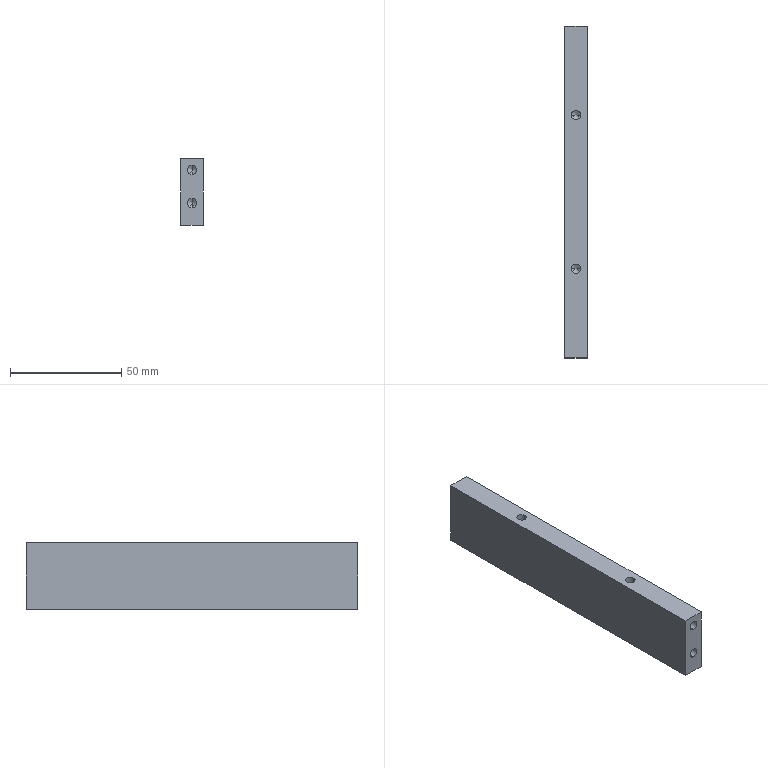Part | STEP file | 05-10 Fixing connection plate 2 | 1 solid | 30 faces | box 10 x 149 x 30 mm | volume 43468 mm3 | cylinder 12 | cone 12 | plane 6 | commonest cylinder face diameters 4.2 x12